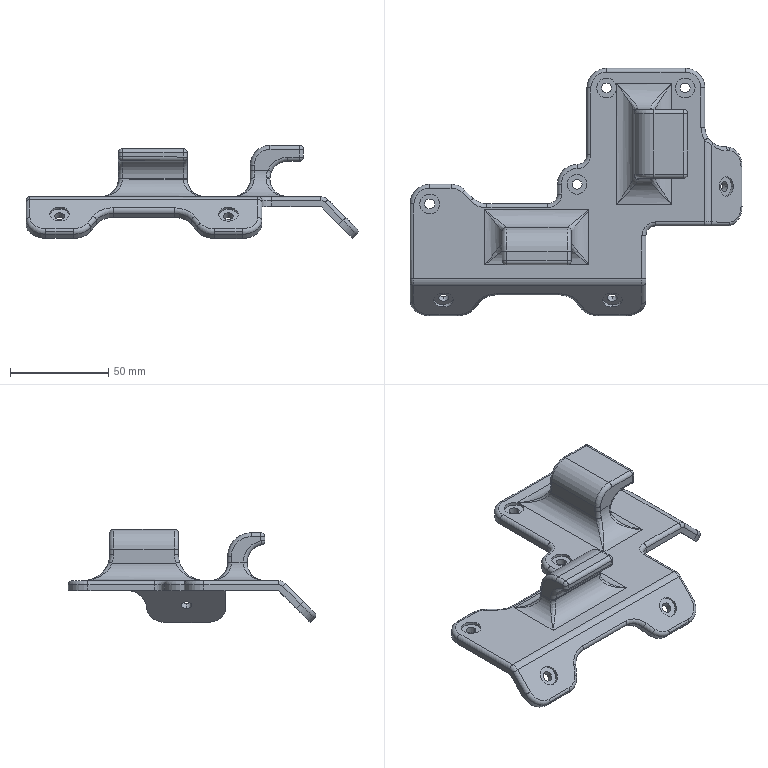Part | SolidWorks | features BaseBody 1 | 1 solid | 206 faces | box 168.914 x 125.853 x 47.37 mm | volume 89409 mm3 | cylinder 108 | plane 44 | torus 33 | spline 13 | sphere 8 | commonest cylinder face diameters 4 x44 10 x19 20 x16 5 x14 18 x8 1 x2